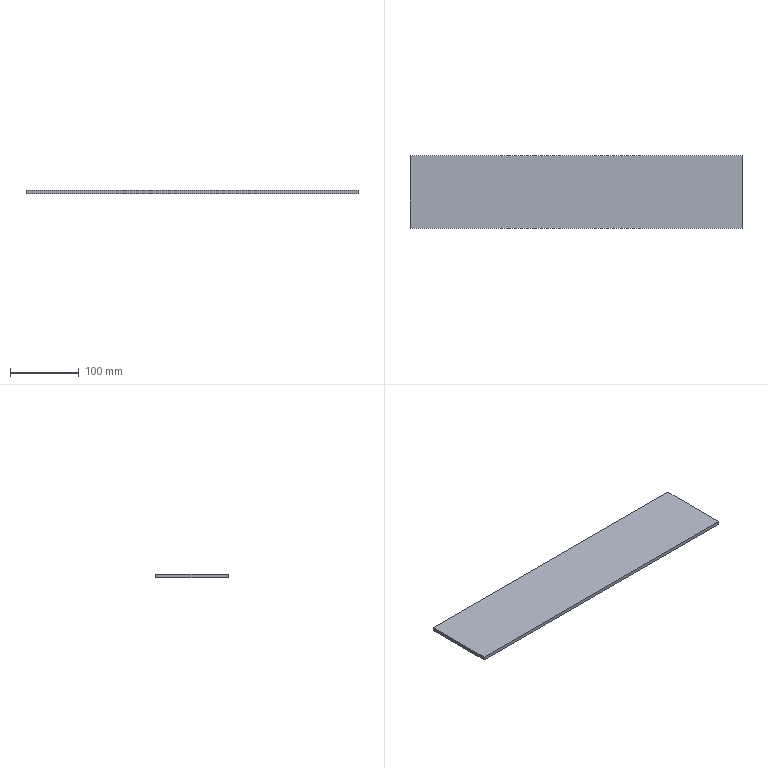Part | SolidWorks | features Extrusion 1, HoleWzd 1 | 1 solid | 6 faces | box 484 x 105 x 5 mm | volume 254100 mm3 | plane 6
STEP:
#1=CARTESIAN_POINT('',(242.,-52.5,0.));
#2=VERTEX_POINT('',#1);
#3=CARTESIAN_POINT('',(242.,52.5,0.));
#4=VERTEX_POINT('',#3);
#5=CARTESIAN_POINT('',(242.,52.5,0.));
#6=DIRECTION('',(0.,1.,0.));
#7=VECTOR('',#6,1000.);
#8=LINE('',#5,#7);
#9=EDGE_CURVE('',#2,#4,#8,.T.);
#10=ORIENTED_EDGE('',*,*,#9,.T.);
#11=CARTESIAN_POINT('',(242.,52.5,5.));
#12=VERTEX_POINT('',#11);
#13=CARTESIAN_POINT('',(242.,52.5,5.));
#14=DIRECTION('',(0.,0.,-1.));
#15=VECTOR('',#14,1000.);
#16=LINE('',#13,#15);
#17=EDGE_CURVE('',#12,#4,#16,.T.);
#18=ORIENTED_EDGE('',*,*,#17,.F.);
#19=CARTESIAN_POINT('',(242.,-52.5,5.));
#20=VERTEX_POINT('',#19);
#21=CARTESIAN_POINT('',(242.,52.5,5.));
#22=DIRECTION('',(0.,1.,0.));
#23=VECTOR('',#22,1000.);
#24=LINE('',#21,#23);
#25=EDGE_CURVE('',#20,#12,#24,.T.);
#26=ORIENTED_EDGE('',*,*,#25,.F.);
#27=CARTESIAN_POINT('',(242.,-52.5,5.));
#28=DIRECTION('',(0.,0.,-1.));
#29=VECTOR('',#28,1000.);
#30=LINE('',#27,#29);
#31=EDGE_CURVE('',#20,#2,#30,.T.);
#32=ORIENTED_EDGE('',*,*,#31,.T.);
#33=EDGE_LOOP('',(#10,#18,#26,#32));
#34=FACE_OUTER_BOUND('',#33,.T.);
#35=CARTESIAN_POINT('',(242.,52.5,5.));
#36=DIRECTION('',(-1.,0.,0.));
#37=DIRECTION('',(0.,0.,1.));
#38=AXIS2_PLACEMENT_3D('',#35,#36,#37);
#39=PLANE('',#38);
#40=ADVANCED_FACE('',(#34),#39,.F.);
#41=CARTESIAN_POINT('',(-242.,52.5,0.));
#42=VERTEX_POINT('',#41);
#43=CARTESIAN_POINT('',(-242.,52.5,0.));
#44=DIRECTION('',(-1.,0.,0.));
#45=VECTOR('',#44,1000.);
#46=LINE('',#43,#45);
#47=EDGE_CURVE('',#4,#42,#46,.T.);
#48=ORIENTED_EDGE('',*,*,#47,.T.);
#49=CARTESIAN_POINT('',(-242.,52.5,5.));
#50=VERTEX_POINT('',#49);
#51=CARTESIAN_POINT('',(-242.,52.5,5.));
#52=DIRECTION('',(0.,0.,-1.));
#53=VECTOR('',#52,1000.);
#54=LINE('',#51,#53);
#55=EDGE_CURVE('',#50,#42,#54,.T.);
#56=ORIENTED_EDGE('',*,*,#55,.F.);
#57=CARTESIAN_POINT('',(-242.,52.5,5.));
#58=DIRECTION('',(-1.,0.,0.));
#59=VECTOR('',#58,1000.);
#60=LINE('',#57,#59);
#61=EDGE_CURVE('',#12,#50,#60,.T.);
#62=ORIENTED_EDGE('',*,*,#61,.F.);
#63=ORIENTED_EDGE('',*,*,#17,.T.);
#64=EDGE_LOOP('',(#48,#56,#62,#63));
#65=FACE_OUTER_BOUND('',#64,.T.);
#66=CARTESIAN_POINT('',(-242.,52.5,5.));
#67=DIRECTION('',(0.,-1.,0.));
#68=DIRECTION('',(0.,0.,-1.));
#69=AXIS2_PLACEMENT_3D('',#66,#67,#68);
#70=PLANE('',#69);
#71=ADVANCED_FACE('',(#65),#70,.F.);
#72=CARTESIAN_POINT('',(-242.,-52.5,0.));
#73=VERTEX_POINT('',#72);
#74=CARTESIAN_POINT('',(-242.,52.5,0.));
#75=DIRECTION('',(0.,-1.,0.));
#76=VECTOR('',#75,1000.);
#77=LINE('',#74,#76);
#78=EDGE_CURVE('',#42,#73,#77,.T.);
#79=ORIENTED_EDGE('',*,*,#78,.T.);
#80=CARTESIAN_POINT('',(-242.,-52.5,5.));
#81=VERTEX_POINT('',#80);
#82=CARTESIAN_POINT('',(-242.,-52.5,5.));
#83=DIRECTION('',(0.,0.,-1.));
#84=VECTOR('',#83,1000.);
#85=LINE('',#82,#84);
#86=EDGE_CURVE('',#81,#73,#85,.T.);
#87=ORIENTED_EDGE('',*,*,#86,.F.);
#88=CARTESIAN_POINT('',(-242.,52.5,5.));
#89=DIRECTION('',(0.,-1.,0.));
#90=VECTOR('',#89,1000.);
#91=LINE('',#88,#90);
#92=EDGE_CURVE('',#50,#81,#91,.T.);
#93=ORIENTED_EDGE('',*,*,#92,.F.);
#94=ORIENTED_EDGE('',*,*,#55,.T.);
#95=EDGE_LOOP('',(#79,#87,#93,#94));
#96=FACE_OUTER_BOUND('',#95,.T.);
#97=CARTESIAN_POINT('',(-242.,52.5,5.));
#98=DIRECTION('',(1.,0.,0.));
#99=DIRECTION('',(0.,0.,-1.));
#100=AXIS2_PLACEMENT_3D('',#97,#98,#99);
#101=PLANE('',#100);
#102=ADVANCED_FACE('',(#96),#101,.F.);
#103=CARTESIAN_POINT('',(-242.,-52.5,0.));
#104=DIRECTION('',(1.,0.,0.));
#105=VECTOR('',#104,1000.);
#106=LINE('',#103,#105);
#107=EDGE_CURVE('',#73,#2,#106,.T.);
#108=ORIENTED_EDGE('',*,*,#107,.T.);
#109=ORIENTED_EDGE('',*,*,#31,.F.);
#110=CARTESIAN_POINT('',(-242.,-52.5,5.));
#111=DIRECTION('',(1.,0.,0.));
#112=VECTOR('',#111,1000.);
#113=LINE('',#110,#112);
#114=EDGE_CURVE('',#81,#20,#113,.T.);
#115=ORIENTED_EDGE('',*,*,#114,.F.);
#116=ORIENTED_EDGE('',*,*,#86,.T.);
#117=EDGE_LOOP('',(#108,#109,#115,#116));
#118=FACE_OUTER_BOUND('',#117,.T.);
#119=CARTESIAN_POINT('',(-242.,-52.5,5.));
#120=DIRECTION('',(0.,1.,0.));
#121=DIRECTION('',(0.,0.,1.));
#122=AXIS2_PLACEMENT_3D('',#119,#120,#121);
#123=PLANE('',#122);
#124=ADVANCED_FACE('',(#118),#123,.F.);
#125=ORIENTED_EDGE('',*,*,#25,.T.);
#126=ORIENTED_EDGE('',*,*,#61,.T.);
#127=ORIENTED_EDGE('',*,*,#92,.T.);
#128=ORIENTED_EDGE('',*,*,#114,.T.);
#129=EDGE_LOOP('',(#125,#126,#127,#128));
#130=FACE_OUTER_BOUND('',#129,.T.);
#131=CARTESIAN_POINT('',(0.,0.,5.));
#132=DIRECTION('',(0.,0.,1.));
#133=DIRECTION('',(1.,0.,0.));
#134=AXIS2_PLACEMENT_3D('',#131,#132,#133);
#135=PLANE('',#134);
#136=ADVANCED_FACE('',(#130),#135,.T.);
#137=ORIENTED_EDGE('',*,*,#9,.F.);
#138=ORIENTED_EDGE('',*,*,#107,.F.);
#139=ORIENTED_EDGE('',*,*,#78,.F.);
#140=ORIENTED_EDGE('',*,*,#47,.F.);
#141=EDGE_LOOP('',(#137,#138,#139,#140));
#142=FACE_OUTER_BOUND('',#141,.T.);
#143=CARTESIAN_POINT('',(0.,0.,0.));
#144=DIRECTION('',(0.,0.,1.));
#145=DIRECTION('',(1.,0.,0.));
#146=AXIS2_PLACEMENT_3D('',#143,#144,#145);
#147=PLANE('',#146);
#148=ADVANCED_FACE('',(#142),#147,.F.);
#149=CLOSED_SHELL('',(#40,#71,#102,#124,#136,#148));
#150=MANIFOLD_SOLID_BREP('',#149);
#151=CARTESIAN_POINT('',(0.,0.,0.));
#152=DIRECTION('',(0.,0.,1.));
#153=DIRECTION('',(1.,0.,0.));
#154=AXIS2_PLACEMENT_3D('',#151,#152,#153);
#155=(LENGTH_UNIT()NAMED_UNIT(*)SI_UNIT(.MILLI.,.METRE.));
#156=UNCERTAINTY_MEASURE_WITH_UNIT(LENGTH_MEASURE(0.00001),#155,'','');
#157=(NAMED_UNIT(*)PLANE_ANGLE_UNIT()SI_UNIT($,.RADIAN.));
#158=(NAMED_UNIT(*)SI_UNIT($,.STERADIAN.)SOLID_ANGLE_UNIT());
#159=(GEOMETRIC_REPRESENTATION_CONTEXT(3)GLOBAL_UNCERTAINTY_ASSIGNED_CONTEXT((#156))GLOBAL_UNIT_ASSIGNED_CONTEXT((#155,#157,#158))REPRESENTATION_CONTEXT('',''));
#160=ADVANCED_BREP_SHAPE_REPRESENTATION('',(#150,#154),#159);